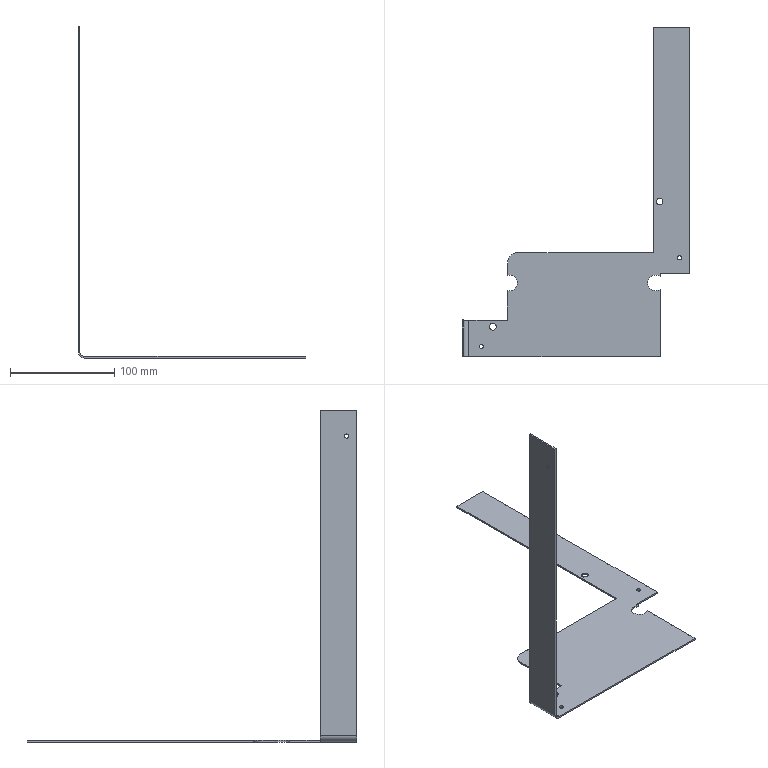Part | SolidWorks | features Cut 6, EdgeFlange 1, Fillet 1, FlatPattern 1, SMBaseFlange 1, SheetMetal 1 | 1 solid | 36 faces | box 218.5 x 316.5 x 318.5 mm | volume 52403 mm3 | plane 20 | cylinder 16 | commonest cylinder face diameters 4 x6 6.4 x4 15 x3 10 x1 13 x1 20 x1
STEP:
#1=CARTESIAN_POINT('',(-99.306,-124.102,-1.5));
#2=VERTEX_POINT('',#1);
#3=CARTESIAN_POINT('',(-108.806,-116.874,-1.5));
#4=VERTEX_POINT('',#3);
#5=CARTESIAN_POINT('',(-106.806,-124.102,-1.5));
#6=DIRECTION('',(0.,0.,1.));
#7=DIRECTION('',(1.,0.,0.));
#8=AXIS2_PLACEMENT_3D('',#5,#6,#7);
#9=CIRCLE('',#8,7.5);
#10=EDGE_CURVE('',#2,#4,#9,.T.);
#11=ORIENTED_EDGE('',*,*,#10,.F.);
#12=CARTESIAN_POINT('',(-99.306,-124.102,0.));
#13=VERTEX_POINT('',#12);
#14=CARTESIAN_POINT('',(-99.306,-124.102,-1.5));
#15=DIRECTION('',(0.,0.,1.));
#16=VECTOR('',#15,1000.);
#17=LINE('',#14,#16);
#18=EDGE_CURVE('',#2,#13,#17,.T.);
#19=ORIENTED_EDGE('',*,*,#18,.T.);
#20=CARTESIAN_POINT('',(-108.806,-116.874,0.));
#21=VERTEX_POINT('',#20);
#22=CARTESIAN_POINT('',(-106.806,-124.102,0.));
#23=DIRECTION('',(0.,0.,1.));
#24=DIRECTION('',(1.,0.,0.));
#25=AXIS2_PLACEMENT_3D('',#22,#23,#24);
#26=CIRCLE('',#25,7.5);
#27=EDGE_CURVE('',#13,#21,#26,.T.);
#28=ORIENTED_EDGE('',*,*,#27,.T.);
#29=CARTESIAN_POINT('',(-108.806,-116.874,-1.5));
#30=DIRECTION('',(0.,0.,1.));
#31=VECTOR('',#30,1000.);
#32=LINE('',#29,#31);
#33=EDGE_CURVE('',#4,#21,#32,.T.);
#34=ORIENTED_EDGE('',*,*,#33,.F.);
#35=EDGE_LOOP('',(#11,#19,#28,#34));
#36=FACE_OUTER_BOUND('',#35,.T.);
#37=CARTESIAN_POINT('',(-106.806,-124.102,-1.5));
#38=DIRECTION('',(0.,0.,1.));
#39=DIRECTION('',(1.,0.,0.));
#40=AXIS2_PLACEMENT_3D('',#37,#38,#39);
#41=CYLINDRICAL_SURFACE('',#40,7.5);
#42=ADVANCED_FACE('',(#36),#41,.F.);
#43=CARTESIAN_POINT('',(-126.006,-166.102,-1.5));
#44=VERTEX_POINT('',#43);
#45=CARTESIAN_POINT('',(-119.606,-166.102,-1.5));
#46=VERTEX_POINT('',#45);
#47=CARTESIAN_POINT('',(-122.806,-166.102,-1.5));
#48=DIRECTION('',(0.,0.,1.));
#49=DIRECTION('',(1.,0.,0.));
#50=AXIS2_PLACEMENT_3D('',#47,#48,#49);
#51=CIRCLE('',#50,3.2);
#52=EDGE_CURVE('',#44,#46,#51,.T.);
#53=ORIENTED_EDGE('',*,*,#52,.F.);
#54=CARTESIAN_POINT('',(-126.006,-166.102,0.));
#55=VERTEX_POINT('',#54);
#56=CARTESIAN_POINT('',(-126.006,-166.102,-1.5));
#57=DIRECTION('',(0.,0.,1.));
#58=VECTOR('',#57,1000.);
#59=LINE('',#56,#58);
#60=EDGE_CURVE('',#44,#55,#59,.T.);
#61=ORIENTED_EDGE('',*,*,#60,.T.);
#62=CARTESIAN_POINT('',(-119.606,-166.102,0.));
#63=VERTEX_POINT('',#62);
#64=CARTESIAN_POINT('',(-122.806,-166.102,0.));
#65=DIRECTION('',(0.,0.,1.));
#66=DIRECTION('',(1.,0.,0.));
#67=AXIS2_PLACEMENT_3D('',#64,#65,#66);
#68=CIRCLE('',#67,3.2);
#69=EDGE_CURVE('',#55,#63,#68,.T.);
#70=ORIENTED_EDGE('',*,*,#69,.T.);
#71=CARTESIAN_POINT('',(-119.606,-166.102,-1.5));
#72=DIRECTION('',(0.,0.,1.));
#73=VECTOR('',#72,1000.);
#74=LINE('',#71,#73);
#75=EDGE_CURVE('',#46,#63,#74,.T.);
#76=ORIENTED_EDGE('',*,*,#75,.F.);
#77=EDGE_LOOP('',(#53,#61,#70,#76));
#78=FACE_OUTER_BOUND('',#77,.T.);
#79=CARTESIAN_POINT('',(-122.806,-166.102,-1.5));
#80=DIRECTION('',(0.,0.,1.));
#81=DIRECTION('',(1.,0.,0.));
#82=AXIS2_PLACEMENT_3D('',#79,#80,#81);
#83=CYLINDRICAL_SURFACE('',#82,3.2);
#84=ADVANCED_FACE('',(#78),#83,.F.);
#85=CARTESIAN_POINT('',(-150.806,-185.102,294.));
#86=VERTEX_POINT('',#85);
#87=CARTESIAN_POINT('',(-150.806,-185.102,290.));
#88=VERTEX_POINT('',#87);
#89=CARTESIAN_POINT('',(-150.806,-185.102,292.));
#90=DIRECTION('',(1.,0.,0.));
#91=DIRECTION('',(0.,0.,-1.));
#92=AXIS2_PLACEMENT_3D('',#89,#90,#91);
#93=CIRCLE('',#92,2.);
#94=EDGE_CURVE('',#86,#88,#93,.T.);
#95=ORIENTED_EDGE('',*,*,#94,.T.);
#96=CARTESIAN_POINT('',(-152.306,-185.102,290.));
#97=VERTEX_POINT('',#96);
#98=CARTESIAN_POINT('',(-142.306,-185.102,290.));
#99=DIRECTION('',(-1.,0.,0.));
#100=VECTOR('',#99,1000.);
#101=LINE('',#98,#100);
#102=EDGE_CURVE('',#88,#97,#101,.T.);
#103=ORIENTED_EDGE('',*,*,#102,.T.);
#104=CARTESIAN_POINT('',(-152.306,-185.102,294.));
#105=VERTEX_POINT('',#104);
#106=CARTESIAN_POINT('',(-152.306,-185.102,292.));
#107=DIRECTION('',(-1.,0.,0.));
#108=DIRECTION('',(0.,0.,1.));
#109=AXIS2_PLACEMENT_3D('',#106,#107,#108);
#110=CIRCLE('',#109,2.);
#111=EDGE_CURVE('',#97,#105,#110,.T.);
#112=ORIENTED_EDGE('',*,*,#111,.T.);
#113=CARTESIAN_POINT('',(-142.306,-185.102,294.));
#114=DIRECTION('',(-1.,0.,0.));
#115=VECTOR('',#114,1000.);
#116=LINE('',#113,#115);
#117=EDGE_CURVE('',#86,#105,#116,.T.);
#118=ORIENTED_EDGE('',*,*,#117,.F.);
#119=EDGE_LOOP('',(#95,#103,#112,#118));
#120=FACE_OUTER_BOUND('',#119,.T.);
#121=CARTESIAN_POINT('',(-142.306,-185.102,292.));
#122=DIRECTION('',(-1.,0.,0.));
#123=DIRECTION('',(0.,0.,1.));
#124=AXIS2_PLACEMENT_3D('',#121,#122,#123);
#125=CYLINDRICAL_SURFACE('',#124,2.);
#126=ADVANCED_FACE('',(#120),#125,.F.);
#127=CARTESIAN_POINT('',(-131.806,-185.102,0.));
#128=VERTEX_POINT('',#127);
#129=CARTESIAN_POINT('',(-135.806,-185.102,0.));
#130=VERTEX_POINT('',#129);
#131=CARTESIAN_POINT('',(-133.806,-185.102,0.));
#132=DIRECTION('',(0.,0.,-1.));
#133=DIRECTION('',(-1.,0.,0.));
#134=AXIS2_PLACEMENT_3D('',#131,#132,#133);
#135=CIRCLE('',#134,2.);
#136=EDGE_CURVE('',#128,#130,#135,.T.);
#137=ORIENTED_EDGE('',*,*,#136,.F.);
#138=CARTESIAN_POINT('',(-131.806,-185.102,-1.5));
#139=VERTEX_POINT('',#138);
#140=CARTESIAN_POINT('',(-131.806,-185.102,8.5));
#141=DIRECTION('',(0.,0.,-1.));
#142=VECTOR('',#141,1000.);
#143=LINE('',#140,#142);
#144=EDGE_CURVE('',#128,#139,#143,.T.);
#145=ORIENTED_EDGE('',*,*,#144,.T.);
#146=CARTESIAN_POINT('',(-135.806,-185.102,-1.5));
#147=VERTEX_POINT('',#146);
#148=CARTESIAN_POINT('',(-133.806,-185.102,-1.5));
#149=DIRECTION('',(0.,0.,-1.));
#150=DIRECTION('',(-1.,0.,0.));
#151=AXIS2_PLACEMENT_3D('',#148,#149,#150);
#152=CIRCLE('',#151,2.);
#153=EDGE_CURVE('',#139,#147,#152,.T.);
#154=ORIENTED_EDGE('',*,*,#153,.T.);
#155=CARTESIAN_POINT('',(-135.806,-185.102,8.5));
#156=DIRECTION('',(0.,0.,-1.));
#157=VECTOR('',#156,1000.);
#158=LINE('',#155,#157);
#159=EDGE_CURVE('',#130,#147,#158,.T.);
#160=ORIENTED_EDGE('',*,*,#159,.F.);
#161=EDGE_LOOP('',(#137,#145,#154,#160));
#162=FACE_OUTER_BOUND('',#161,.T.);
#163=CARTESIAN_POINT('',(-133.806,-185.102,8.5));
#164=DIRECTION('',(0.,0.,-1.));
#165=DIRECTION('',(-1.,0.,0.));
#166=AXIS2_PLACEMENT_3D('',#163,#164,#165);
#167=CYLINDRICAL_SURFACE('',#166,2.);
#168=ADVANCED_FACE('',(#162),#167,.F.);
#169=CARTESIAN_POINT('',(58.194,-100.102,0.));
#170=VERTEX_POINT('',#169);
#171=CARTESIAN_POINT('',(54.194,-100.102,0.));
#172=VERTEX_POINT('',#171);
#173=CARTESIAN_POINT('',(56.194,-100.102,0.));
#174=DIRECTION('',(0.,0.,-1.));
#175=DIRECTION('',(-1.,0.,0.));
#176=AXIS2_PLACEMENT_3D('',#173,#174,#175);
#177=CIRCLE('',#176,2.);
#178=EDGE_CURVE('',#170,#172,#177,.T.);
#179=ORIENTED_EDGE('',*,*,#178,.F.);
#180=CARTESIAN_POINT('',(58.194,-100.102,-1.5));
#181=VERTEX_POINT('',#180);
#182=CARTESIAN_POINT('',(58.194,-100.102,8.5));
#183=DIRECTION('',(0.,0.,-1.));
#184=VECTOR('',#183,1000.);
#185=LINE('',#182,#184);
#186=EDGE_CURVE('',#170,#181,#185,.T.);
#187=ORIENTED_EDGE('',*,*,#186,.T.);
#188=CARTESIAN_POINT('',(54.194,-100.102,-1.5));
#189=VERTEX_POINT('',#188);
#190=CARTESIAN_POINT('',(56.194,-100.102,-1.5));
#191=DIRECTION('',(0.,0.,-1.));
#192=DIRECTION('',(-1.,0.,0.));
#193=AXIS2_PLACEMENT_3D('',#190,#191,#192);
#194=CIRCLE('',#193,2.);
#195=EDGE_CURVE('',#181,#189,#194,.T.);
#196=ORIENTED_EDGE('',*,*,#195,.T.);
#197=CARTESIAN_POINT('',(54.194,-100.102,8.5));
#198=DIRECTION('',(0.,0.,-1.));
#199=VECTOR('',#198,1000.);
#200=LINE('',#197,#199);
#201=EDGE_CURVE('',#172,#189,#200,.T.);
#202=ORIENTED_EDGE('',*,*,#201,.F.);
#203=EDGE_LOOP('',(#179,#187,#196,#202));
#204=FACE_OUTER_BOUND('',#203,.T.);
#205=CARTESIAN_POINT('',(56.194,-100.102,8.5));
#206=DIRECTION('',(0.,0.,-1.));
#207=DIRECTION('',(-1.,0.,0.));
#208=AXIS2_PLACEMENT_3D('',#205,#206,#207);
#209=CYLINDRICAL_SURFACE('',#208,2.);
#210=ADVANCED_FACE('',(#204),#209,.F.);
#211=CARTESIAN_POINT('',(40.394,-46.102,0.));
#212=VERTEX_POINT('',#211);
#213=CARTESIAN_POINT('',(33.994,-46.102,0.));
#214=VERTEX_POINT('',#213);
#215=CARTESIAN_POINT('',(37.194,-46.102,0.));
#216=DIRECTION('',(0.,0.,-1.));
#217=DIRECTION('',(-1.,0.,0.));
#218=AXIS2_PLACEMENT_3D('',#215,#216,#217);
#219=CIRCLE('',#218,3.2);
#220=EDGE_CURVE('',#212,#214,#219,.T.);
#221=ORIENTED_EDGE('',*,*,#220,.F.);
#222=CARTESIAN_POINT('',(40.394,-46.102,-1.5));
#223=VERTEX_POINT('',#222);
#224=CARTESIAN_POINT('',(40.394,-46.102,8.5));
#225=DIRECTION('',(0.,0.,-1.));
#226=VECTOR('',#225,1000.);
#227=LINE('',#224,#226);
#228=EDGE_CURVE('',#212,#223,#227,.T.);
#229=ORIENTED_EDGE('',*,*,#228,.T.);
#230=CARTESIAN_POINT('',(33.994,-46.102,-1.5));
#231=VERTEX_POINT('',#230);
#232=CARTESIAN_POINT('',(37.194,-46.102,-1.5));
#233=DIRECTION('',(0.,0.,-1.));
#234=DIRECTION('',(-1.,0.,0.));
#235=AXIS2_PLACEMENT_3D('',#232,#233,#234);
#236=CIRCLE('',#235,3.2);
#237=EDGE_CURVE('',#223,#231,#236,.T.);
#238=ORIENTED_EDGE('',*,*,#237,.T.);
#239=CARTESIAN_POINT('',(33.994,-46.102,8.5));
#240=DIRECTION('',(0.,0.,-1.));
#241=VECTOR('',#240,1000.);
#242=LINE('',#239,#241);
#243=EDGE_CURVE('',#214,#231,#242,.T.);
#244=ORIENTED_EDGE('',*,*,#243,.F.);
#245=EDGE_LOOP('',(#221,#229,#238,#244));
#246=FACE_OUTER_BOUND('',#245,.T.);
#247=CARTESIAN_POINT('',(37.194,-46.102,8.5));
#248=DIRECTION('',(0.,0.,-1.));
#249=DIRECTION('',(-1.,0.,0.));
#250=AXIS2_PLACEMENT_3D('',#247,#248,#249);
#251=CYLINDRICAL_SURFACE('',#250,3.2);
#252=ADVANCED_FACE('',(#246),#251,.F.);
#253=CARTESIAN_POINT('',(37.694,-118.102,0.));
#254=VERTEX_POINT('',#253);
#255=CARTESIAN_POINT('',(37.694,-115.102,0.));
#256=VERTEX_POINT('',#255);
#257=CARTESIAN_POINT('',(37.694,-195.102,0.));
#258=DIRECTION('',(0.,1.,0.));
#259=VECTOR('',#258,1000.);
#260=LINE('',#257,#259);
#261=EDGE_CURVE('',#254,#256,#260,.T.);
#262=ORIENTED_EDGE('',*,*,#261,.F.);
#263=CARTESIAN_POINT('',(37.694,-118.102,-1.5));
#264=VERTEX_POINT('',#263);
#265=CARTESIAN_POINT('',(37.694,-118.102,-1.5));
#266=DIRECTION('',(0.,0.,1.));
#267=VECTOR('',#266,1000.);
#268=LINE('',#265,#267);
#269=EDGE_CURVE('',#264,#254,#268,.T.);
#270=ORIENTED_EDGE('',*,*,#269,.F.);
#271=CARTESIAN_POINT('',(37.694,-115.102,-1.5));
#272=VERTEX_POINT('',#271);
#273=CARTESIAN_POINT('',(37.694,-195.102,-1.5));
#274=DIRECTION('',(0.,1.,0.));
#275=VECTOR('',#274,1000.);
#276=LINE('',#273,#275);
#277=EDGE_CURVE('',#264,#272,#276,.T.);
#278=ORIENTED_EDGE('',*,*,#277,.T.);
#279=CARTESIAN_POINT('',(37.694,-115.102,-1.5));
#280=DIRECTION('',(0.,0.,1.));
#281=VECTOR('',#280,1000.);
#282=LINE('',#279,#281);
#283=EDGE_CURVE('',#272,#256,#282,.T.);
#284=ORIENTED_EDGE('',*,*,#283,.T.);
#285=EDGE_LOOP('',(#262,#270,#278,#284));
#286=FACE_OUTER_BOUND('',#285,.T.);
#287=CARTESIAN_POINT('',(37.694,-195.102,-1.5));
#288=DIRECTION('',(1.,0.,0.));
#289=DIRECTION('',(0.,0.,-1.));
#290=AXIS2_PLACEMENT_3D('',#287,#288,#289);
#291=PLANE('',#290);
#292=ADVANCED_FACE('',(#286),#291,.T.);
#293=CARTESIAN_POINT('',(37.694,-195.102,-1.5));
#294=VERTEX_POINT('',#293);
#295=CARTESIAN_POINT('',(37.694,-130.102,-1.5));
#296=VERTEX_POINT('',#295);
#297=CARTESIAN_POINT('',(37.694,-195.102,-1.5));
#298=DIRECTION('',(0.,1.,0.));
#299=VECTOR('',#298,1000.);
#300=LINE('',#297,#299);
#301=EDGE_CURVE('',#294,#296,#300,.T.);
#302=ORIENTED_EDGE('',*,*,#301,.T.);
#303=CARTESIAN_POINT('',(37.694,-130.102,0.));
#304=VERTEX_POINT('',#303);
#305=CARTESIAN_POINT('',(37.694,-130.102,-1.5));
#306=DIRECTION('',(0.,0.,1.));
#307=VECTOR('',#306,1000.);
#308=LINE('',#305,#307);
#309=EDGE_CURVE('',#296,#304,#308,.T.);
#310=ORIENTED_EDGE('',*,*,#309,.T.);
#311=CARTESIAN_POINT('',(37.694,-195.102,0.));
#312=VERTEX_POINT('',#311);
#313=CARTESIAN_POINT('',(37.694,-195.102,0.));
#314=DIRECTION('',(0.,1.,0.));
#315=VECTOR('',#314,1000.);
#316=LINE('',#313,#315);
#317=EDGE_CURVE('',#312,#304,#316,.T.);
#318=ORIENTED_EDGE('',*,*,#317,.F.);
#319=CARTESIAN_POINT('',(37.694,-195.102,-1.5));
#320=DIRECTION('',(0.,0.,1.));
#321=VECTOR('',#320,1000.);
#322=LINE('',#319,#321);
#323=EDGE_CURVE('',#294,#312,#322,.T.);
#324=ORIENTED_EDGE('',*,*,#323,.F.);
#325=EDGE_LOOP('',(#302,#310,#318,#324));
#326=FACE_OUTER_BOUND('',#325,.T.);
#327=CARTESIAN_POINT('',(37.694,-195.102,-1.5));
#328=DIRECTION('',(1.,0.,0.));
#329=DIRECTION('',(0.,0.,-1.));
#330=AXIS2_PLACEMENT_3D('',#327,#328,#329);
#331=PLANE('',#330);
#332=ADVANCED_FACE('',(#326),#331,.T.);
#333=CARTESIAN_POINT('',(-108.806,-131.331,0.));
#334=VERTEX_POINT('',#333);
#335=CARTESIAN_POINT('',(-108.806,-160.102,0.));
#336=VERTEX_POINT('',#335);
#337=CARTESIAN_POINT('',(-108.806,-95.102,0.));
#338=DIRECTION('',(0.,-1.,0.));
#339=VECTOR('',#338,1000.);
#340=LINE('',#337,#339);
#341=EDGE_CURVE('',#334,#336,#340,.T.);
#342=ORIENTED_EDGE('',*,*,#341,.F.);
#343=CARTESIAN_POINT('',(-108.806,-131.331,-1.5));
#344=VERTEX_POINT('',#343);
#345=CARTESIAN_POINT('',(-108.806,-131.331,-1.5));
#346=DIRECTION('',(0.,0.,1.));
#347=VECTOR('',#346,1000.);
#348=LINE('',#345,#347);
#349=EDGE_CURVE('',#344,#334,#348,.T.);
#350=ORIENTED_EDGE('',*,*,#349,.F.);
#351=CARTESIAN_POINT('',(-108.806,-160.102,-1.5));
#352=VERTEX_POINT('',#351);
#353=CARTESIAN_POINT('',(-108.806,-95.102,-1.5));
#354=DIRECTION('',(0.,-1.,0.));
#355=VECTOR('',#354,1000.);
#356=LINE('',#353,#355);
#357=EDGE_CURVE('',#344,#352,#356,.T.);
#358=ORIENTED_EDGE('',*,*,#357,.T.);
#359=CARTESIAN_POINT('',(-108.806,-160.102,-1.5));
#360=DIRECTION('',(0.,0.,1.));
#361=VECTOR('',#360,1000.);
#362=LINE('',#359,#361);
#363=EDGE_CURVE('',#352,#336,#362,.T.);
#364=ORIENTED_EDGE('',*,*,#363,.T.);
#365=EDGE_LOOP('',(#342,#350,#358,#364));
#366=FACE_OUTER_BOUND('',#365,.T.);
#367=CARTESIAN_POINT('',(-108.806,-95.102,-1.5));
#368=DIRECTION('',(-1.,0.,0.));
#369=DIRECTION('',(0.,-1.,0.));
#370=AXIS2_PLACEMENT_3D('',#367,#368,#369);
#371=PLANE('',#370);
#372=ADVANCED_FACE('',(#366),#371,.T.);
#373=CARTESIAN_POINT('',(-108.806,-105.102,-1.5));
#374=VERTEX_POINT('',#373);
#375=CARTESIAN_POINT('',(-108.806,-95.102,-1.5));
#376=DIRECTION('',(0.,-1.,0.));
#377=VECTOR('',#376,1000.);
#378=LINE('',#375,#377);
#379=EDGE_CURVE('',#374,#4,#378,.T.);
#380=ORIENTED_EDGE('',*,*,#379,.T.);
#381=ORIENTED_EDGE('',*,*,#33,.T.);
#382=CARTESIAN_POINT('',(-108.806,-105.102,0.));
#383=VERTEX_POINT('',#382);
#384=CARTESIAN_POINT('',(-108.806,-95.102,0.));
#385=DIRECTION('',(0.,-1.,0.));
#386=VECTOR('',#385,1000.);
#387=LINE('',#384,#386);
#388=EDGE_CURVE('',#383,#21,#387,.T.);
#389=ORIENTED_EDGE('',*,*,#388,.F.);
#390=CARTESIAN_POINT('',(-108.806,-105.102,-1.5));
#391=DIRECTION('',(0.,0.,-1.));
#392=VECTOR('',#391,1000.);
#393=LINE('',#390,#392);
#394=EDGE_CURVE('',#383,#374,#393,.T.);
#395=ORIENTED_EDGE('',*,*,#394,.T.);
#396=EDGE_LOOP('',(#380,#381,#389,#395));
#397=FACE_OUTER_BOUND('',#396,.T.);
#398=CARTESIAN_POINT('',(-108.806,-95.102,-1.5));
#399=DIRECTION('',(-1.,0.,0.));
#400=DIRECTION('',(0.,-1.,0.));
#401=AXIS2_PLACEMENT_3D('',#398,#399,#400);
#402=PLANE('',#401);
#403=ADVANCED_FACE('',(#397),#402,.T.);
#404=CARTESIAN_POINT('',(-145.806,-195.102,0.));
#405=VERTEX_POINT('',#404);
#406=CARTESIAN_POINT('',(-152.306,-195.102,0.));
#407=DIRECTION('',(1.,0.,0.));
#408=VECTOR('',#407,1000.);
#409=LINE('',#406,#408);
#410=EDGE_CURVE('',#405,#312,#409,.T.);
#411=ORIENTED_EDGE('',*,*,#410,.F.);
#412=CARTESIAN_POINT('',(-145.806,-195.102,-1.5));
#413=VERTEX_POINT('',#412);
#414=CARTESIAN_POINT('',(-145.806,-195.102,0.));
#415=DIRECTION('',(0.,0.,-1.));
#416=VECTOR('',#415,1000.);
#417=LINE('',#414,#416);
#418=EDGE_CURVE('',#405,#413,#417,.T.);
#419=ORIENTED_EDGE('',*,*,#418,.T.);
#420=CARTESIAN_POINT('',(-152.306,-195.102,-1.5));
#421=DIRECTION('',(1.,0.,0.));
#422=VECTOR('',#421,1000.);
#423=LINE('',#420,#422);
#424=EDGE_CURVE('',#413,#294,#423,.T.);
#425=ORIENTED_EDGE('',*,*,#424,.T.);
#426=ORIENTED_EDGE('',*,*,#323,.T.);
#427=EDGE_LOOP('',(#411,#419,#425,#426));
#428=FACE_OUTER_BOUND('',#427,.T.);
#429=CARTESIAN_POINT('',(-152.306,-195.102,-1.5));
#430=DIRECTION('',(0.,-1.,0.));
#431=DIRECTION('',(0.,0.,-1.));
#432=AXIS2_PLACEMENT_3D('',#429,#430,#431);
#433=PLANE('',#432);
#434=ADVANCED_FACE('',(#428),#433,.T.);
#435=CARTESIAN_POINT('',(-122.806,-166.102,-1.5));
#436=DIRECTION('',(0.,0.,1.));
#437=DIRECTION('',(1.,0.,0.));
#438=AXIS2_PLACEMENT_3D('',#435,#436,#437);
#439=CIRCLE('',#438,3.2);
#440=EDGE_CURVE('',#46,#44,#439,.T.);
#441=ORIENTED_EDGE('',*,*,#440,.T.);
#442=ORIENTED_EDGE('',*,*,#52,.T.);
#443=EDGE_LOOP('',(#441,#442));
#444=FACE_BOUND('',#443,.T.);
#445=CARTESIAN_POINT('',(-133.806,-185.102,-1.5));
#446=DIRECTION('',(0.,0.,-1.));
#447=DIRECTION('',(-1.,0.,0.));
#448=AXIS2_PLACEMENT_3D('',#445,#446,#447);
#449=CIRCLE('',#448,2.);
#450=EDGE_CURVE('',#147,#139,#449,.T.);
#451=ORIENTED_EDGE('',*,*,#450,.F.);
#452=ORIENTED_EDGE('',*,*,#153,.F.);
#453=EDGE_LOOP('',(#451,#452));
#454=FACE_BOUND('',#453,.T.);
#455=CARTESIAN_POINT('',(56.194,-100.102,-1.5));
#456=DIRECTION('',(0.,0.,-1.));
#457=DIRECTION('',(-1.,0.,0.));
#458=AXIS2_PLACEMENT_3D('',#455,#456,#457);
#459=CIRCLE('',#458,2.);
#460=EDGE_CURVE('',#189,#181,#459,.T.);
#461=ORIENTED_EDGE('',*,*,#460,.F.);
#462=ORIENTED_EDGE('',*,*,#195,.F.);
#463=EDGE_LOOP('',(#461,#462));
#464=FACE_BOUND('',#463,.T.);
#465=CARTESIAN_POINT('',(37.194,-46.102,-1.5));
#466=DIRECTION('',(0.,0.,-1.));
#467=DIRECTION('',(-1.,0.,0.));
#468=AXIS2_PLACEMENT_3D('',#465,#466,#467);
#469=CIRCLE('',#468,3.2);
#470=EDGE_CURVE('',#231,#223,#469,.T.);
#471=ORIENTED_EDGE('',*,*,#470,.F.);
#472=ORIENTED_EDGE('',*,*,#237,.F.);
#473=EDGE_LOOP('',(#471,#472));
#474=FACE_BOUND('',#473,.T.);
#475=ORIENTED_EDGE('',*,*,#277,.F.);
#476=CARTESIAN_POINT('',(33.194,-124.102,-1.5));
#477=DIRECTION('',(0.,0.,1.));
#478=DIRECTION('',(1.,0.,0.));
#479=AXIS2_PLACEMENT_3D('',#476,#477,#478);
#480=CIRCLE('',#479,7.5);
#481=EDGE_CURVE('',#264,#296,#480,.T.);
#482=ORIENTED_EDGE('',*,*,#481,.T.);
#483=ORIENTED_EDGE('',*,*,#301,.F.);
#484=ORIENTED_EDGE('',*,*,#424,.F.);
#485=CARTESIAN_POINT('',(-145.806,-160.102,-1.5));
#486=VERTEX_POINT('',#485);
#487=CARTESIAN_POINT('',(-145.806,-195.102,-1.5));
#488=DIRECTION('',(0.,1.,0.));
#489=VECTOR('',#488,1000.);
#490=LINE('',#487,#489);
#491=EDGE_CURVE('',#413,#486,#490,.T.);
#492=ORIENTED_EDGE('',*,*,#491,.T.);
#493=CARTESIAN_POINT('',(-108.806,-160.102,-1.5));
#494=DIRECTION('',(-1.,0.,0.));
#495=VECTOR('',#494,1000.);
#496=LINE('',#493,#495);
#497=EDGE_CURVE('',#352,#486,#496,.T.);
#498=ORIENTED_EDGE('',*,*,#497,.F.);
#499=ORIENTED_EDGE('',*,*,#357,.F.);
#500=CARTESIAN_POINT('',(-106.806,-124.102,-1.5));
#501=DIRECTION('',(0.,0.,1.));
#502=DIRECTION('',(1.,0.,0.));
#503=AXIS2_PLACEMENT_3D('',#500,#501,#502);
#504=CIRCLE('',#503,7.5);
#505=EDGE_CURVE('',#344,#2,#504,.T.);
#506=ORIENTED_EDGE('',*,*,#505,.T.);
#507=ORIENTED_EDGE('',*,*,#10,.T.);
#508=ORIENTED_EDGE('',*,*,#379,.F.);
#509=CARTESIAN_POINT('',(-98.806,-95.102,-1.5));
#510=VERTEX_POINT('',#509);
#511=CARTESIAN_POINT('',(-98.806,-105.102,-1.5));
#512=DIRECTION('',(0.,0.,-1.));
#513=DIRECTION('',(-1.,0.,0.));
#514=AXIS2_PLACEMENT_3D('',#511,#512,#513);
#515=CIRCLE('',#514,10.);
#516=EDGE_CURVE('',#374,#510,#515,.T.);
#517=ORIENTED_EDGE('',*,*,#516,.T.);
#518=CARTESIAN_POINT('',(31.194,-95.102,-1.5));
#519=VERTEX_POINT('',#518);
#520=CARTESIAN_POINT('',(-108.806,-95.102,-1.5));
#521=DIRECTION('',(-1.,0.,0.));
#522=VECTOR('',#521,1000.);
#523=LINE('',#520,#522);
#524=EDGE_CURVE('',#519,#510,#523,.T.);
#525=ORIENTED_EDGE('',*,*,#524,.F.);
#526=CARTESIAN_POINT('',(31.194,121.398,-1.5));
#527=VERTEX_POINT('',#526);
#528=CARTESIAN_POINT('',(31.194,121.398,-1.5));
#529=DIRECTION('',(0.,-1.,0.));
#530=VECTOR('',#529,1000.);
#531=LINE('',#528,#530);
#532=EDGE_CURVE('',#527,#519,#531,.T.);
#533=ORIENTED_EDGE('',*,*,#532,.F.);
#534=CARTESIAN_POINT('',(66.194,121.398,-1.5));
#535=VERTEX_POINT('',#534);
#536=CARTESIAN_POINT('',(31.194,121.398,-1.5));
#537=DIRECTION('',(-1.,0.,0.));
#538=VECTOR('',#537,1000.);
#539=LINE('',#536,#538);
#540=EDGE_CURVE('',#535,#527,#539,.T.);
#541=ORIENTED_EDGE('',*,*,#540,.F.);
#542=CARTESIAN_POINT('',(66.194,-115.102,-1.5));
#543=VERTEX_POINT('',#542);
#544=CARTESIAN_POINT('',(66.194,121.398,-1.5));
#545=DIRECTION('',(0.,1.,0.));
#546=VECTOR('',#545,1000.);
#547=LINE('',#544,#546);
#548=EDGE_CURVE('',#543,#535,#547,.T.);
#549=ORIENTED_EDGE('',*,*,#548,.F.);
#550=CARTESIAN_POINT('',(37.694,-115.102,-1.5));
#551=DIRECTION('',(1.,0.,0.));
#552=VECTOR('',#551,1000.);
#553=LINE('',#550,#552);
#554=EDGE_CURVE('',#272,#543,#553,.T.);
#555=ORIENTED_EDGE('',*,*,#554,.F.);
#556=EDGE_LOOP('',(#475,#482,#483,#484,#492,#498,#499,#506,#507,#508,#517,#525,#533,#541,#549,#555));
#557=FACE_OUTER_BOUND('',#556,.T.);
#558=CARTESIAN_POINT('',(0.,0.,-1.5));
#559=DIRECTION('',(0.,0.,-1.));
#560=DIRECTION('',(-1.,0.,0.));
#561=AXIS2_PLACEMENT_3D('',#558,#559,#560);
#562=PLANE('',#561);
#563=ADVANCED_FACE('',(#444,#454,#464,#474,#557),#562,.T.);
#564=CARTESIAN_POINT('',(33.194,-124.102,0.));
#565=DIRECTION('',(0.,0.,1.));
#566=DIRECTION('',(1.,0.,0.));
#567=AXIS2_PLACEMENT_3D('',#564,#565,#566);
#568=CIRCLE('',#567,7.5);
#569=EDGE_CURVE('',#254,#304,#568,.T.);
#570=ORIENTED_EDGE('',*,*,#569,.F.);
#571=ORIENTED_EDGE('',*,*,#261,.T.);
#572=CARTESIAN_POINT('',(66.194,-115.102,0.));
#573=VERTEX_POINT('',#572);
#574=CARTESIAN_POINT('',(37.694,-115.102,0.));
#575=DIRECTION('',(1.,0.,0.));
#576=VECTOR('',#575,1000.);
#577=LINE('',#574,#576);
#578=EDGE_CURVE('',#256,#573,#577,.T.);
#579=ORIENTED_EDGE('',*,*,#578,.T.);
#580=CARTESIAN_POINT('',(66.194,121.398,0.));
#581=VERTEX_POINT('',#580);
#582=CARTESIAN_POINT('',(66.194,121.398,0.));
#583=DIRECTION('',(0.,1.,0.));
#584=VECTOR('',#583,1000.);
#585=LINE('',#582,#584);
#586=EDGE_CURVE('',#573,#581,#585,.T.);
#587=ORIENTED_EDGE('',*,*,#586,.T.);
#588=CARTESIAN_POINT('',(31.194,121.398,0.));
#589=VERTEX_POINT('',#588);
#590=CARTESIAN_POINT('',(31.194,121.398,0.));
#591=DIRECTION('',(-1.,0.,0.));
#592=VECTOR('',#591,1000.);
#593=LINE('',#590,#592);
#594=EDGE_CURVE('',#581,#589,#593,.T.);
#595=ORIENTED_EDGE('',*,*,#594,.T.);
#596=CARTESIAN_POINT('',(31.194,-95.102,0.));
#597=VERTEX_POINT('',#596);
#598=CARTESIAN_POINT('',(31.194,121.398,0.));
#599=DIRECTION('',(0.,-1.,0.));
#600=VECTOR('',#599,1000.);
#601=LINE('',#598,#600);
#602=EDGE_CURVE('',#589,#597,#601,.T.);
#603=ORIENTED_EDGE('',*,*,#602,.T.);
#604=CARTESIAN_POINT('',(-98.806,-95.102,0.));
#605=VERTEX_POINT('',#604);
#606=CARTESIAN_POINT('',(-108.806,-95.102,0.));
#607=DIRECTION('',(-1.,0.,0.));
#608=VECTOR('',#607,1000.);
#609=LINE('',#606,#608);
#610=EDGE_CURVE('',#597,#605,#609,.T.);
#611=ORIENTED_EDGE('',*,*,#610,.T.);
#612=CARTESIAN_POINT('',(-98.806,-105.102,0.));
#613=DIRECTION('',(0.,0.,1.));
#614=DIRECTION('',(-1.,0.,0.));
#615=AXIS2_PLACEMENT_3D('',#612,#613,#614);
#616=CIRCLE('',#615,10.);
#617=EDGE_CURVE('',#605,#383,#616,.T.);
#618=ORIENTED_EDGE('',*,*,#617,.T.);
#619=ORIENTED_EDGE('',*,*,#388,.T.);
#620=ORIENTED_EDGE('',*,*,#27,.F.);
#621=CARTESIAN_POINT('',(-106.806,-124.102,0.));
#622=DIRECTION('',(0.,0.,1.));
#623=DIRECTION('',(1.,0.,0.));
#624=AXIS2_PLACEMENT_3D('',#621,#622,#623);
#625=CIRCLE('',#624,7.5);
#626=EDGE_CURVE('',#334,#13,#625,.T.);
#627=ORIENTED_EDGE('',*,*,#626,.F.);
#628=ORIENTED_EDGE('',*,*,#341,.T.);
#629=CARTESIAN_POINT('',(-145.806,-160.102,0.));
#630=VERTEX_POINT('',#629);
#631=CARTESIAN_POINT('',(-108.806,-160.102,0.));
#632=DIRECTION('',(-1.,0.,0.));
#633=VECTOR('',#632,1000.);
#634=LINE('',#631,#633);
#635=EDGE_CURVE('',#336,#630,#634,.T.);
#636=ORIENTED_EDGE('',*,*,#635,.T.);
#637=CARTESIAN_POINT('',(-145.806,-195.102,0.));
#638=DIRECTION('',(0.,1.,0.));
#639=VECTOR('',#638,1000.);
#640=LINE('',#637,#639);
#641=EDGE_CURVE('',#405,#630,#640,.T.);
#642=ORIENTED_EDGE('',*,*,#641,.F.);
#643=ORIENTED_EDGE('',*,*,#410,.T.);
#644=ORIENTED_EDGE('',*,*,#317,.T.);
#645=EDGE_LOOP('',(#570,#571,#579,#587,#595,#603,#611,#618,#619,#620,#627,#628,#636,#642,#643,#644));
#646=FACE_OUTER_BOUND('',#645,.T.);
#647=CARTESIAN_POINT('',(-122.806,-166.102,0.));
#648=DIRECTION('',(0.,0.,1.));
#649=DIRECTION('',(1.,0.,0.));
#650=AXIS2_PLACEMENT_3D('',#647,#648,#649);
#651=CIRCLE('',#650,3.2);
#652=EDGE_CURVE('',#63,#55,#651,.T.);
#653=ORIENTED_EDGE('',*,*,#652,.F.);
#654=ORIENTED_EDGE('',*,*,#69,.F.);
#655=EDGE_LOOP('',(#653,#654));
#656=FACE_BOUND('',#655,.T.);
#657=CARTESIAN_POINT('',(-133.806,-185.102,0.));
#658=DIRECTION('',(0.,0.,-1.));
#659=DIRECTION('',(-1.,0.,0.));
#660=AXIS2_PLACEMENT_3D('',#657,#658,#659);
#661=CIRCLE('',#660,2.);
#662=EDGE_CURVE('',#130,#128,#661,.T.);
#663=ORIENTED_EDGE('',*,*,#662,.T.);
#664=ORIENTED_EDGE('',*,*,#136,.T.);
#665=EDGE_LOOP('',(#663,#664));
#666=FACE_BOUND('',#665,.T.);
#667=CARTESIAN_POINT('',(56.194,-100.102,0.));
#668=DIRECTION('',(0.,0.,-1.));
#669=DIRECTION('',(-1.,0.,0.));
#670=AXIS2_PLACEMENT_3D('',#667,#668,#669);
#671=CIRCLE('',#670,2.);
#672=EDGE_CURVE('',#172,#170,#671,.T.);
#673=ORIENTED_EDGE('',*,*,#672,.T.);
#674=ORIENTED_EDGE('',*,*,#178,.T.);
#675=EDGE_LOOP('',(#673,#674));
#676=FACE_BOUND('',#675,.T.);
#677=CARTESIAN_POINT('',(37.194,-46.102,0.));
#678=DIRECTION('',(0.,0.,-1.));
#679=DIRECTION('',(-1.,0.,0.));
#680=AXIS2_PLACEMENT_3D('',#677,#678,#679);
#681=CIRCLE('',#680,3.2);
#682=EDGE_CURVE('',#214,#212,#681,.T.);
#683=ORIENTED_EDGE('',*,*,#682,.T.);
#684=ORIENTED_EDGE('',*,*,#220,.T.);
#685=EDGE_LOOP('',(#683,#684));
#686=FACE_BOUND('',#685,.T.);
#687=CARTESIAN_POINT('',(0.,0.,0.));
#688=DIRECTION('',(0.,0.,-1.));
#689=DIRECTION('',(-1.,0.,0.));
#690=AXIS2_PLACEMENT_3D('',#687,#688,#689);
#691=PLANE('',#690);
#692=ADVANCED_FACE('',(#646,#656,#666,#676,#686),#691,.F.);
#693=ORIENTED_EDGE('',*,*,#594,.F.);
#694=CARTESIAN_POINT('',(66.194,121.398,-1.5));
#695=DIRECTION('',(0.,0.,1.));
#696=VECTOR('',#695,1000.);
#697=LINE('',#694,#696);
#698=EDGE_CURVE('',#535,#581,#697,.T.);
#699=ORIENTED_EDGE('',*,*,#698,.F.);
#700=ORIENTED_EDGE('',*,*,#540,.T.);
#701=CARTESIAN_POINT('',(31.194,121.398,-1.5));
#702=DIRECTION('',(0.,0.,1.));
#703=VECTOR('',#702,1000.);
#704=LINE('',#701,#703);
#705=EDGE_CURVE('',#527,#589,#704,.T.);
#706=ORIENTED_EDGE('',*,*,#705,.T.);
#707=EDGE_LOOP('',(#693,#699,#700,#706));
#708=FACE_OUTER_BOUND('',#707,.T.);
#709=CARTESIAN_POINT('',(31.194,121.398,-1.5));
#710=DIRECTION('',(0.,1.,0.));
#711=DIRECTION('',(0.,0.,1.));
#712=AXIS2_PLACEMENT_3D('',#709,#710,#711);
#713=PLANE('',#712);
#714=ADVANCED_FACE('',(#708),#713,.T.);
#715=ORIENTED_EDGE('',*,*,#586,.F.);
#716=CARTESIAN_POINT('',(66.194,-115.102,-1.5));
#717=DIRECTION('',(0.,0.,1.));
#718=VECTOR('',#717,1000.);
#719=LINE('',#716,#718);
#720=EDGE_CURVE('',#543,#573,#719,.T.);
#721=ORIENTED_EDGE('',*,*,#720,.F.);
#722=ORIENTED_EDGE('',*,*,#548,.T.);
#723=ORIENTED_EDGE('',*,*,#698,.T.);
#724=EDGE_LOOP('',(#715,#721,#722,#723));
#725=FACE_OUTER_BOUND('',#724,.T.);
#726=CARTESIAN_POINT('',(66.194,121.398,-1.5));
#727=DIRECTION('',(1.,0.,0.));
#728=DIRECTION('',(0.,1.,0.));
#729=AXIS2_PLACEMENT_3D('',#726,#727,#728);
#730=PLANE('',#729);
#731=ADVANCED_FACE('',(#725),#730,.T.);
#732=ORIENTED_EDGE('',*,*,#578,.F.);
#733=ORIENTED_EDGE('',*,*,#283,.F.);
#734=ORIENTED_EDGE('',*,*,#554,.T.);
#735=ORIENTED_EDGE('',*,*,#720,.T.);
#736=EDGE_LOOP('',(#732,#733,#734,#735));
#737=FACE_OUTER_BOUND('',#736,.T.);
#738=CARTESIAN_POINT('',(37.694,-115.102,-1.5));
#739=DIRECTION('',(0.,-1.,0.));
#740=DIRECTION('',(0.,0.,-1.));
#741=AXIS2_PLACEMENT_3D('',#738,#739,#740);
#742=PLANE('',#741);
#743=ADVANCED_FACE('',(#737),#742,.T.);
#744=CARTESIAN_POINT('',(-145.806,-160.102,0.));
#745=DIRECTION('',(0.,0.,-1.));
#746=VECTOR('',#745,1000.);
#747=LINE('',#744,#746);
#748=EDGE_CURVE('',#630,#486,#747,.T.);
#749=ORIENTED_EDGE('',*,*,#748,.F.);
#750=ORIENTED_EDGE('',*,*,#635,.F.);
#751=ORIENTED_EDGE('',*,*,#363,.F.);
#752=ORIENTED_EDGE('',*,*,#497,.T.);
#753=EDGE_LOOP('',(#749,#750,#751,#752));
#754=FACE_OUTER_BOUND('',#753,.T.);
#755=CARTESIAN_POINT('',(-108.806,-160.102,-1.5));
#756=DIRECTION('',(0.,1.,0.));
#757=DIRECTION('',(-1.,0.,0.));
#758=AXIS2_PLACEMENT_3D('',#755,#756,#757);
#759=PLANE('',#758);
#760=ADVANCED_FACE('',(#754),#759,.T.);
#761=ORIENTED_EDGE('',*,*,#524,.T.);
#762=CARTESIAN_POINT('',(-98.806,-95.102,-1.5));
#763=DIRECTION('',(0.,0.,1.));
#764=VECTOR('',#763,1000.);
#765=LINE('',#762,#764);
#766=EDGE_CURVE('',#510,#605,#765,.T.);
#767=ORIENTED_EDGE('',*,*,#766,.T.);
#768=ORIENTED_EDGE('',*,*,#610,.F.);
#769=CARTESIAN_POINT('',(31.194,-95.102,-1.5));
#770=DIRECTION('',(0.,0.,1.));
#771=VECTOR('',#770,1000.);
#772=LINE('',#769,#771);
#773=EDGE_CURVE('',#519,#597,#772,.T.);
#774=ORIENTED_EDGE('',*,*,#773,.F.);
#775=EDGE_LOOP('',(#761,#767,#768,#774));
#776=FACE_OUTER_BOUND('',#775,.T.);
#777=CARTESIAN_POINT('',(-108.806,-95.102,-1.5));
#778=DIRECTION('',(0.,1.,0.));
#779=DIRECTION('',(-1.,0.,0.));
#780=AXIS2_PLACEMENT_3D('',#777,#778,#779);
#781=PLANE('',#780);
#782=ADVANCED_FACE('',(#776),#781,.T.);
#783=ORIENTED_EDGE('',*,*,#602,.F.);
#784=ORIENTED_EDGE('',*,*,#705,.F.);
#785=ORIENTED_EDGE('',*,*,#532,.T.);
#786=ORIENTED_EDGE('',*,*,#773,.T.);
#787=EDGE_LOOP('',(#783,#784,#785,#786));
#788=FACE_OUTER_BOUND('',#787,.T.);
#789=CARTESIAN_POINT('',(31.194,121.398,-1.5));
#790=DIRECTION('',(-1.,0.,0.));
#791=DIRECTION('',(0.,-1.,0.));
#792=AXIS2_PLACEMENT_3D('',#789,#790,#791);
#793=PLANE('',#792);
#794=ADVANCED_FACE('',(#788),#793,.T.);
#795=CARTESIAN_POINT('',(-150.806,-160.102,5.));
#796=VERTEX_POINT('',#795);
#797=CARTESIAN_POINT('',(-152.306,-160.102,5.));
#798=VERTEX_POINT('',#797);
#799=CARTESIAN_POINT('',(-152.306,-160.102,5.));
#800=DIRECTION('',(-1.,0.,0.));
#801=VECTOR('',#800,1000.);
#802=LINE('',#799,#801);
#803=EDGE_CURVE('',#796,#798,#802,.T.);
#804=ORIENTED_EDGE('',*,*,#803,.F.);
#805=CARTESIAN_POINT('',(-145.806,-160.102,5.));
#806=DIRECTION('',(0.,1.,0.));
#807=DIRECTION('',(0.,0.,-1.));
#808=AXIS2_PLACEMENT_3D('',#805,#806,#807);
#809=CIRCLE('',#808,5.);
#810=EDGE_CURVE('',#630,#796,#809,.T.);
#811=ORIENTED_EDGE('',*,*,#810,.F.);
#812=ORIENTED_EDGE('',*,*,#748,.T.);
#813=CARTESIAN_POINT('',(-145.806,-160.102,5.));
#814=DIRECTION('',(0.,1.,0.));
#815=DIRECTION('',(0.,0.,-1.));
#816=AXIS2_PLACEMENT_3D('',#813,#814,#815);
#817=CIRCLE('',#816,6.5);
#818=EDGE_CURVE('',#486,#798,#817,.T.);
#819=ORIENTED_EDGE('',*,*,#818,.T.);
#820=EDGE_LOOP('',(#804,#811,#812,#819));
#821=FACE_OUTER_BOUND('',#820,.T.);
#822=CARTESIAN_POINT('',(-145.806,-160.102,5.));
#823=DIRECTION('',(0.,1.,0.));
#824=DIRECTION('',(0.,0.,1.));
#825=AXIS2_PLACEMENT_3D('',#822,#823,#824);
#826=PLANE('',#825);
#827=ADVANCED_FACE('',(#821),#826,.T.);
#828=CARTESIAN_POINT('',(-150.806,-195.102,5.));
#829=VERTEX_POINT('',#828);
#830=CARTESIAN_POINT('',(-145.806,-195.102,5.));
#831=DIRECTION('',(0.,-1.,0.));
#832=DIRECTION('',(0.,0.,-1.));
#833=AXIS2_PLACEMENT_3D('',#830,#831,#832);
#834=CIRCLE('',#833,5.);
#835=EDGE_CURVE('',#829,#405,#834,.T.);
#836=ORIENTED_EDGE('',*,*,#835,.F.);
#837=CARTESIAN_POINT('',(-152.306,-195.102,5.));
#838=VERTEX_POINT('',#837);
#839=CARTESIAN_POINT('',(-150.806,-195.102,5.));
#840=DIRECTION('',(-1.,0.,0.));
#841=VECTOR('',#840,1000.);
#842=LINE('',#839,#841);
#843=EDGE_CURVE('',#829,#838,#842,.T.);
#844=ORIENTED_EDGE('',*,*,#843,.T.);
#845=CARTESIAN_POINT('',(-145.806,-195.102,5.));
#846=DIRECTION('',(0.,-1.,0.));
#847=DIRECTION('',(0.,0.,-1.));
#848=AXIS2_PLACEMENT_3D('',#845,#846,#847);
#849=CIRCLE('',#848,6.5);
#850=EDGE_CURVE('',#838,#413,#849,.T.);
#851=ORIENTED_EDGE('',*,*,#850,.T.);
#852=ORIENTED_EDGE('',*,*,#418,.F.);
#853=EDGE_LOOP('',(#836,#844,#851,#852));
#854=FACE_OUTER_BOUND('',#853,.T.);
#855=CARTESIAN_POINT('',(-145.806,-195.102,5.));
#856=DIRECTION('',(0.,1.,0.));
#857=DIRECTION('',(0.,0.,1.));
#858=AXIS2_PLACEMENT_3D('',#855,#856,#857);
#859=PLANE('',#858);
#860=ADVANCED_FACE('',(#854),#859,.F.);
#861=ORIENTED_EDGE('',*,*,#491,.F.);
#862=ORIENTED_EDGE('',*,*,#850,.F.);
#863=CARTESIAN_POINT('',(-152.306,-160.102,5.));
#864=DIRECTION('',(0.,1.,0.));
#865=VECTOR('',#864,1000.);
#866=LINE('',#863,#865);
#867=EDGE_CURVE('',#838,#798,#866,.T.);
#868=ORIENTED_EDGE('',*,*,#867,.T.);
#869=ORIENTED_EDGE('',*,*,#818,.F.);
#870=EDGE_LOOP('',(#861,#862,#868,#869));
#871=FACE_OUTER_BOUND('',#870,.T.);
#872=CARTESIAN_POINT('',(-145.806,-195.102,5.));
#873=DIRECTION('',(0.,-1.,0.));
#874=DIRECTION('',(-1.,0.,0.));
#875=AXIS2_PLACEMENT_3D('',#872,#873,#874);
#876=CYLINDRICAL_SURFACE('',#875,6.5);
#877=ADVANCED_FACE('',(#871),#876,.T.);
#878=ORIENTED_EDGE('',*,*,#641,.T.);
#879=ORIENTED_EDGE('',*,*,#810,.T.);
#880=CARTESIAN_POINT('',(-150.806,-160.102,5.));
#881=DIRECTION('',(0.,-1.,0.));
#882=VECTOR('',#881,1000.);
#883=LINE('',#880,#882);
#884=EDGE_CURVE('',#796,#829,#883,.T.);
#885=ORIENTED_EDGE('',*,*,#884,.T.);
#886=ORIENTED_EDGE('',*,*,#835,.T.);
#887=EDGE_LOOP('',(#878,#879,#885,#886));
#888=FACE_OUTER_BOUND('',#887,.T.);
#889=CARTESIAN_POINT('',(-145.806,-195.102,5.));
#890=DIRECTION('',(0.,-1.,0.));
#891=DIRECTION('',(-1.,0.,0.));
#892=AXIS2_PLACEMENT_3D('',#889,#890,#891);
#893=CYLINDRICAL_SURFACE('',#892,5.);
#894=ADVANCED_FACE('',(#888),#893,.F.);
#895=ORIENTED_EDGE('',*,*,#843,.F.);
#896=CARTESIAN_POINT('',(-150.806,-195.102,317.));
#897=VERTEX_POINT('',#896);
#898=CARTESIAN_POINT('',(-150.806,-195.102,317.));
#899=DIRECTION('',(0.,0.,1.));
#900=VECTOR('',#899,1000.);
#901=LINE('',#898,#900);
#902=EDGE_CURVE('',#829,#897,#901,.T.);
#903=ORIENTED_EDGE('',*,*,#902,.T.);
#904=CARTESIAN_POINT('',(-152.306,-195.102,317.));
#905=VERTEX_POINT('',#904);
#906=CARTESIAN_POINT('',(-152.306,-195.102,317.));
#907=DIRECTION('',(1.,0.,0.));
#908=VECTOR('',#907,1000.);
#909=LINE('',#906,#908);
#910=EDGE_CURVE('',#905,#897,#909,.T.);
#911=ORIENTED_EDGE('',*,*,#910,.F.);
#912=CARTESIAN_POINT('',(-152.306,-195.102,0.));
#913=DIRECTION('',(0.,0.,1.));
#914=VECTOR('',#913,1000.);
#915=LINE('',#912,#914);
#916=EDGE_CURVE('',#838,#905,#915,.T.);
#917=ORIENTED_EDGE('',*,*,#916,.F.);
#918=EDGE_LOOP('',(#895,#903,#911,#917));
#919=FACE_OUTER_BOUND('',#918,.T.);
#920=CARTESIAN_POINT('',(-152.306,-195.102,317.));
#921=DIRECTION('',(0.,1.,0.));
#922=DIRECTION('',(0.,0.,1.));
#923=AXIS2_PLACEMENT_3D('',#920,#921,#922);
#924=PLANE('',#923);
#925=ADVANCED_FACE('',(#919),#924,.F.);
#926=ORIENTED_EDGE('',*,*,#803,.T.);
#927=CARTESIAN_POINT('',(-152.306,-160.102,317.));
#928=VERTEX_POINT('',#927);
#929=CARTESIAN_POINT('',(-152.306,-160.102,0.));
#930=DIRECTION('',(0.,0.,-1.));
#931=VECTOR('',#930,1000.);
#932=LINE('',#929,#931);
#933=EDGE_CURVE('',#928,#798,#932,.T.);
#934=ORIENTED_EDGE('',*,*,#933,.F.);
#935=CARTESIAN_POINT('',(-150.806,-160.102,317.));
#936=VERTEX_POINT('',#935);
#937=CARTESIAN_POINT('',(-152.306,-160.102,317.));
#938=DIRECTION('',(1.,0.,0.));
#939=VECTOR('',#938,1000.);
#940=LINE('',#937,#939);
#941=EDGE_CURVE('',#928,#936,#940,.T.);
#942=ORIENTED_EDGE('',*,*,#941,.T.);
#943=CARTESIAN_POINT('',(-150.806,-160.102,0.));
#944=DIRECTION('',(0.,0.,-1.));
#945=VECTOR('',#944,1000.);
#946=LINE('',#943,#945);
#947=EDGE_CURVE('',#936,#796,#946,.T.);
#948=ORIENTED_EDGE('',*,*,#947,.T.);
#949=EDGE_LOOP('',(#926,#934,#942,#948));
#950=FACE_OUTER_BOUND('',#949,.T.);
#951=CARTESIAN_POINT('',(-152.306,-160.102,0.));
#952=DIRECTION('',(0.,-1.,0.));
#953=DIRECTION('',(0.,0.,-1.));
#954=AXIS2_PLACEMENT_3D('',#951,#952,#953);
#955=PLANE('',#954);
#956=ADVANCED_FACE('',(#950),#955,.F.);
#957=CARTESIAN_POINT('',(-152.306,-185.102,292.));
#958=DIRECTION('',(-1.,0.,0.));
#959=DIRECTION('',(0.,0.,1.));
#960=AXIS2_PLACEMENT_3D('',#957,#958,#959);
#961=CIRCLE('',#960,2.);
#962=EDGE_CURVE('',#105,#97,#961,.T.);
#963=ORIENTED_EDGE('',*,*,#962,.F.);
#964=ORIENTED_EDGE('',*,*,#111,.F.);
#965=EDGE_LOOP('',(#963,#964));
#966=FACE_BOUND('',#965,.T.);
#967=ORIENTED_EDGE('',*,*,#867,.F.);
#968=ORIENTED_EDGE('',*,*,#916,.T.);
#969=CARTESIAN_POINT('',(-152.306,0.,317.));
#970=DIRECTION('',(0.,1.,0.));
#971=VECTOR('',#970,1000.);
#972=LINE('',#969,#971);
#973=EDGE_CURVE('',#905,#928,#972,.T.);
#974=ORIENTED_EDGE('',*,*,#973,.T.);
#975=ORIENTED_EDGE('',*,*,#933,.T.);
#976=EDGE_LOOP('',(#967,#968,#974,#975));
#977=FACE_OUTER_BOUND('',#976,.T.);
#978=CARTESIAN_POINT('',(-152.306,0.,0.));
#979=DIRECTION('',(1.,0.,0.));
#980=DIRECTION('',(0.,0.,-1.));
#981=AXIS2_PLACEMENT_3D('',#978,#979,#980);
#982=PLANE('',#981);
#983=ADVANCED_FACE('',(#966,#977),#982,.F.);
#984=ORIENTED_EDGE('',*,*,#94,.F.);
#985=CARTESIAN_POINT('',(-150.806,-185.102,292.));
#986=DIRECTION('',(1.,0.,0.));
#987=DIRECTION('',(0.,0.,-1.));
#988=AXIS2_PLACEMENT_3D('',#985,#986,#987);
#989=CIRCLE('',#988,2.);
#990=EDGE_CURVE('',#88,#86,#989,.T.);
#991=ORIENTED_EDGE('',*,*,#990,.F.);
#992=EDGE_LOOP('',(#984,#991));
#993=FACE_BOUND('',#992,.T.);
#994=ORIENTED_EDGE('',*,*,#902,.F.);
#995=ORIENTED_EDGE('',*,*,#884,.F.);
#996=ORIENTED_EDGE('',*,*,#947,.F.);
#997=CARTESIAN_POINT('',(-150.806,-160.102,317.));
#998=DIRECTION('',(0.,1.,0.));
#999=VECTOR('',#998,1000.);
#1000=LINE('',#997,#999);
#1001=EDGE_CURVE('',#897,#936,#1000,.T.);
#1002=ORIENTED_EDGE('',*,*,#1001,.F.);
#1003=EDGE_LOOP('',(#994,#995,#996,#1002));
#1004=FACE_OUTER_BOUND('',#1003,.T.);
#1005=CARTESIAN_POINT('',(-150.806,0.,0.));
#1006=DIRECTION('',(1.,0.,0.));
#1007=DIRECTION('',(0.,0.,-1.));
#1008=AXIS2_PLACEMENT_3D('',#1005,#1006,#1007);
#1009=PLANE('',#1008);
#1010=ADVANCED_FACE('',(#993,#1004),#1009,.T.);
#1011=ORIENTED_EDGE('',*,*,#1001,.T.);
#1012=ORIENTED_EDGE('',*,*,#941,.F.);
#1013=ORIENTED_EDGE('',*,*,#973,.F.);
#1014=ORIENTED_EDGE('',*,*,#910,.T.);
#1015=EDGE_LOOP('',(#1011,#1012,#1013,#1014));
#1016=FACE_OUTER_BOUND('',#1015,.T.);
#1017=CARTESIAN_POINT('',(-152.306,-160.102,317.));
#1018=DIRECTION('',(0.,0.,-1.));
#1019=DIRECTION('',(-1.,0.,0.));
#1020=AXIS2_PLACEMENT_3D('',#1017,#1018,#1019);
#1021=PLANE('',#1020);
#1022=ADVANCED_FACE('',(#1016),#1021,.F.);
#1023=ORIENTED_EDGE('',*,*,#516,.F.);
#1024=ORIENTED_EDGE('',*,*,#394,.F.);
#1025=ORIENTED_EDGE('',*,*,#617,.F.);
#1026=ORIENTED_EDGE('',*,*,#766,.F.);
#1027=EDGE_LOOP('',(#1023,#1024,#1025,#1026));
#1028=FACE_OUTER_BOUND('',#1027,.T.);
#1029=CARTESIAN_POINT('',(-98.806,-105.102,-1.5));
#1030=DIRECTION('',(0.,0.,1.));
#1031=DIRECTION('',(1.,0.,0.));
#1032=AXIS2_PLACEMENT_3D('',#1029,#1030,#1031);
#1033=CYLINDRICAL_SURFACE('',#1032,10.);
#1034=ADVANCED_FACE('',(#1028),#1033,.T.);
#1035=ORIENTED_EDGE('',*,*,#228,.F.);
#1036=ORIENTED_EDGE('',*,*,#682,.F.);
#1037=ORIENTED_EDGE('',*,*,#243,.T.);
#1038=ORIENTED_EDGE('',*,*,#470,.T.);
#1039=EDGE_LOOP('',(#1035,#1036,#1037,#1038));
#1040=FACE_OUTER_BOUND('',#1039,.T.);
#1041=CARTESIAN_POINT('',(37.194,-46.102,8.5));
#1042=DIRECTION('',(0.,0.,-1.));
#1043=DIRECTION('',(-1.,0.,0.));
#1044=AXIS2_PLACEMENT_3D('',#1041,#1042,#1043);
#1045=CYLINDRICAL_SURFACE('',#1044,3.2);
#1046=ADVANCED_FACE('',(#1040),#1045,.F.);
#1047=ORIENTED_EDGE('',*,*,#186,.F.);
#1048=ORIENTED_EDGE('',*,*,#672,.F.);
#1049=ORIENTED_EDGE('',*,*,#201,.T.);
#1050=ORIENTED_EDGE('',*,*,#460,.T.);
#1051=EDGE_LOOP('',(#1047,#1048,#1049,#1050));
#1052=FACE_OUTER_BOUND('',#1051,.T.);
#1053=CARTESIAN_POINT('',(56.194,-100.102,8.5));
#1054=DIRECTION('',(0.,0.,-1.));
#1055=DIRECTION('',(-1.,0.,0.));
#1056=AXIS2_PLACEMENT_3D('',#1053,#1054,#1055);
#1057=CYLINDRICAL_SURFACE('',#1056,2.);
#1058=ADVANCED_FACE('',(#1052),#1057,.F.);
#1059=ORIENTED_EDGE('',*,*,#144,.F.);
#1060=ORIENTED_EDGE('',*,*,#662,.F.);
#1061=ORIENTED_EDGE('',*,*,#159,.T.);
#1062=ORIENTED_EDGE('',*,*,#450,.T.);
#1063=EDGE_LOOP('',(#1059,#1060,#1061,#1062));
#1064=FACE_OUTER_BOUND('',#1063,.T.);
#1065=CARTESIAN_POINT('',(-133.806,-185.102,8.5));
#1066=DIRECTION('',(0.,0.,-1.));
#1067=DIRECTION('',(-1.,0.,0.));
#1068=AXIS2_PLACEMENT_3D('',#1065,#1066,#1067);
#1069=CYLINDRICAL_SURFACE('',#1068,2.);
#1070=ADVANCED_FACE('',(#1064),#1069,.F.);
#1071=ORIENTED_EDGE('',*,*,#102,.F.);
#1072=ORIENTED_EDGE('',*,*,#990,.T.);
#1073=ORIENTED_EDGE('',*,*,#117,.T.);
#1074=ORIENTED_EDGE('',*,*,#962,.T.);
#1075=EDGE_LOOP('',(#1071,#1072,#1073,#1074));
#1076=FACE_OUTER_BOUND('',#1075,.T.);
#1077=CARTESIAN_POINT('',(-142.306,-185.102,292.));
#1078=DIRECTION('',(-1.,0.,0.));
#1079=DIRECTION('',(0.,0.,1.));
#1080=AXIS2_PLACEMENT_3D('',#1077,#1078,#1079);
#1081=CYLINDRICAL_SURFACE('',#1080,2.);
#1082=ADVANCED_FACE('',(#1076),#1081,.F.);
#1083=ORIENTED_EDGE('',*,*,#60,.F.);
#1084=ORIENTED_EDGE('',*,*,#440,.F.);
#1085=ORIENTED_EDGE('',*,*,#75,.T.);
#1086=ORIENTED_EDGE('',*,*,#652,.T.);
#1087=EDGE_LOOP('',(#1083,#1084,#1085,#1086));
#1088=FACE_OUTER_BOUND('',#1087,.T.);
#1089=CARTESIAN_POINT('',(-122.806,-166.102,-1.5));
#1090=DIRECTION('',(0.,0.,1.));
#1091=DIRECTION('',(1.,0.,0.));
#1092=AXIS2_PLACEMENT_3D('',#1089,#1090,#1091);
#1093=CYLINDRICAL_SURFACE('',#1092,3.2);
#1094=ADVANCED_FACE('',(#1088),#1093,.F.);
#1095=ORIENTED_EDGE('',*,*,#18,.F.);
#1096=ORIENTED_EDGE('',*,*,#505,.F.);
#1097=ORIENTED_EDGE('',*,*,#349,.T.);
#1098=ORIENTED_EDGE('',*,*,#626,.T.);
#1099=EDGE_LOOP('',(#1095,#1096,#1097,#1098));
#1100=FACE_OUTER_BOUND('',#1099,.T.);
#1101=CARTESIAN_POINT('',(-106.806,-124.102,-1.5));
#1102=DIRECTION('',(0.,0.,1.));
#1103=DIRECTION('',(1.,0.,0.));
#1104=AXIS2_PLACEMENT_3D('',#1101,#1102,#1103);
#1105=CYLINDRICAL_SURFACE('',#1104,7.5);
#1106=ADVANCED_FACE('',(#1100),#1105,.F.);
#1107=ORIENTED_EDGE('',*,*,#481,.F.);
#1108=ORIENTED_EDGE('',*,*,#269,.T.);
#1109=ORIENTED_EDGE('',*,*,#569,.T.);
#1110=ORIENTED_EDGE('',*,*,#309,.F.);
#1111=EDGE_LOOP('',(#1107,#1108,#1109,#1110));
#1112=FACE_OUTER_BOUND('',#1111,.T.);
#1113=CARTESIAN_POINT('',(33.194,-124.102,-1.5));
#1114=DIRECTION('',(0.,0.,1.));
#1115=DIRECTION('',(1.,0.,0.));
#1116=AXIS2_PLACEMENT_3D('',#1113,#1114,#1115);
#1117=CYLINDRICAL_SURFACE('',#1116,7.5);
#1118=ADVANCED_FACE('',(#1112),#1117,.F.);
#1119=CLOSED_SHELL('',(#42,#84,#126,#168,#210,#252,#292,#332,#372,#403,#434,#563,#692,#714,#731,#743,#760,#782,#794,#827,#860,#877,#894,#925,#956,#983,#1010,#1022,#1034,#1046,#1058,#1070,#1082,#1094,#1106,#1118));
#1120=MANIFOLD_SOLID_BREP('',#1119);
#1121=CARTESIAN_POINT('',(0.,0.,0.));
#1122=DIRECTION('',(0.,0.,1.));
#1123=DIRECTION('',(1.,0.,0.));
#1124=AXIS2_PLACEMENT_3D('',#1121,#1122,#1123);
#1125=(LENGTH_UNIT()NAMED_UNIT(*)SI_UNIT(.MILLI.,.METRE.));
#1126=UNCERTAINTY_MEASURE_WITH_UNIT(LENGTH_MEASURE(0.00001),#1125,'','');
#1127=(NAMED_UNIT(*)PLANE_ANGLE_UNIT()SI_UNIT($,.RADIAN.));
#1128=(NAMED_UNIT(*)SI_UNIT($,.STERADIAN.)SOLID_ANGLE_UNIT());
#1129=(GEOMETRIC_REPRESENTATION_CONTEXT(3)GLOBAL_UNCERTAINTY_ASSIGNED_CONTEXT((#1126))GLOBAL_UNIT_ASSIGNED_CONTEXT((#1125,#1127,#1128))REPRESENTATION_CONTEXT('',''));
#1130=ADVANCED_BREP_SHAPE_REPRESENTATION('',(#1120,#1124),#1129);